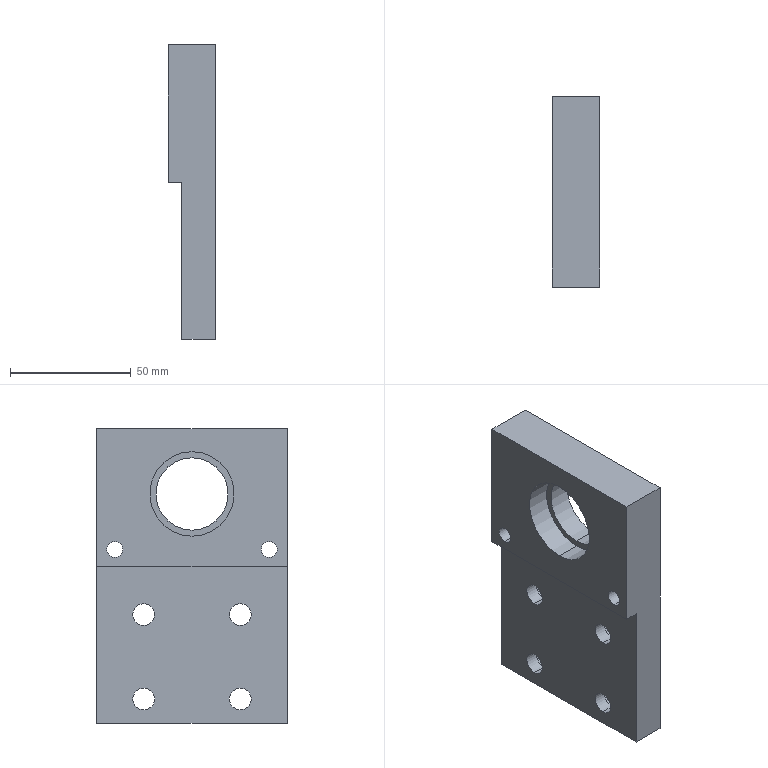Part | STEP file | PN_0023 (connecting plate) | 1 solid | 43 faces | box 19.5 x 79 x 122 mm | volume 133748 mm3 | cylinder 28 | plane 15 | commonest cylinder face diameters 9 x8 15 x8 6.6 x4 11 x4 30 x2 35 x2